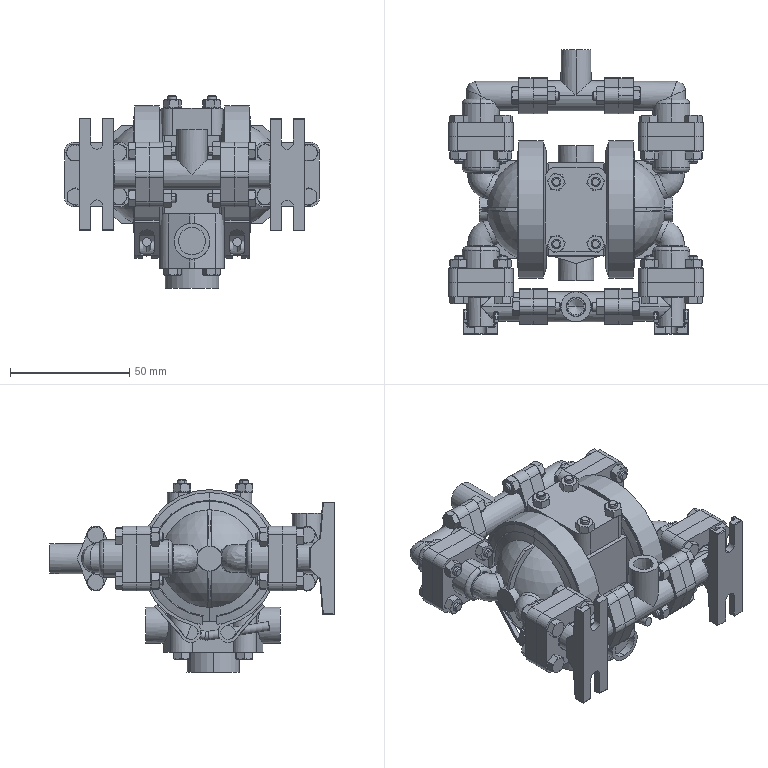Part | NX | 71 solids | 2147 faces | box 106.8 x 119.1 x 80.79 mm | volume 246955 mm3 | plane 766 | cone 710 | cylinder 537 | torus 64 | sphere 40 | spline 30 | commonest cylinder face diameters 3.81 x112 0.6 x108 7.2 x72 3.063 x56 6 x34 11.4 x24